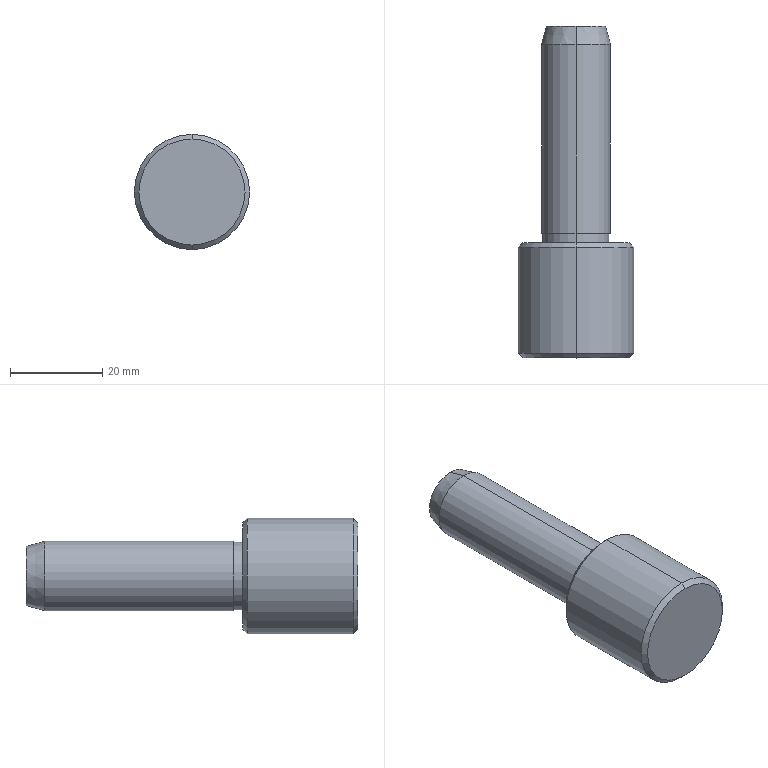Part | STEP file | OP10-024_fix-pin | 1 solid | 16 faces | box 25 x 72 x 25 mm | volume 20386 mm3 | cone 6 | cylinder 6 | plane 4 | commonest cylinder face diameters 14.6 x2 15 x2 25 x2
STEP:
#1=CARTESIAN_POINT('',(0.,0.,0.));
#2=DIRECTION('',(0.,0.,1.));
#3=DIRECTION('',(1.,0.,0.));
#4=AXIS2_PLACEMENT_3D('',#1,#2,#3);
#5=CARTESIAN_POINT('',(0.,72.,6.428));
#6=VERTEX_POINT('',#5);
#7=CARTESIAN_POINT('',(0.,72.,-6.428));
#8=VERTEX_POINT('',#7);
#9=CARTESIAN_POINT('',(0.,72.,0.));
#10=DIRECTION('',(0.,1.,0.));
#11=DIRECTION('',(0.,0.,1.));
#12=AXIS2_PLACEMENT_3D('',#9,#10,#11);
#13=CIRCLE('',#12,6.428);
#14=CARTESIAN_POINT('',(0.,72.,0.));
#15=DIRECTION('',(0.,-1.,0.));
#16=DIRECTION('',(0.,0.,-1.));
#17=AXIS2_PLACEMENT_3D('',#14,#15,#16);
#18=CONICAL_SURFACE('',#17,6.428,0.2618);
#19=CARTESIAN_POINT('',(3.142,0.));
#20=DIRECTION('',(-1.,0.));
#21=VECTOR('',#20,1.);
#22=LINE('',#19,#21);
#23=(GEOMETRIC_REPRESENTATION_CONTEXT(2)PARAMETRIC_REPRESENTATION_CONTEXT()REPRESENTATION_CONTEXT('',''));
#24=DEFINITIONAL_REPRESENTATION('',(#22),#23);
#25=PCURVE('',#18,#24);
#26=CARTESIAN_POINT('',(0.,72.,0.));
#27=DIRECTION('',(0.,1.,0.));
#28=DIRECTION('',(0.,0.,1.));
#29=AXIS2_PLACEMENT_3D('',#26,#27,#28);
#30=PLANE('',#29);
#31=CARTESIAN_POINT('',(0.,0.));
#32=DIRECTION('',(1.,0.));
#33=AXIS2_PLACEMENT_2D('',#31,#32);
#34=CIRCLE('',#33,6.428);
#35=(GEOMETRIC_REPRESENTATION_CONTEXT(2)PARAMETRIC_REPRESENTATION_CONTEXT()REPRESENTATION_CONTEXT('',''));
#36=DEFINITIONAL_REPRESENTATION('',(#34),#35);
#37=PCURVE('',#30,#36);
#38=SURFACE_CURVE('',#13,(#25,#37),.PCURVE_S1.);
#39=EDGE_CURVE('',#6,#8,#38,.T.);
#40=ORIENTED_EDGE('',*,*,#39,.F.);
#41=CARTESIAN_POINT('',(0.,68.,7.5));
#42=VERTEX_POINT('',#41);
#43=CARTESIAN_POINT('',(0.,72.,6.428));
#44=DIRECTION('',(0.,-0.9659,0.2588));
#45=VECTOR('',#44,1.);
#46=LINE('',#43,#45);
#47=CARTESIAN_POINT('',(3.142,0.));
#48=DIRECTION('',(0.,1.));
#49=VECTOR('',#48,1.);
#50=LINE('',#47,#49);
#51=(GEOMETRIC_REPRESENTATION_CONTEXT(2)PARAMETRIC_REPRESENTATION_CONTEXT()REPRESENTATION_CONTEXT('',''));
#52=DEFINITIONAL_REPRESENTATION('',(#50),#51);
#53=PCURVE('',#18,#52);
#54=CARTESIAN_POINT('',(0.,72.,0.));
#55=DIRECTION('',(0.,-1.,0.));
#56=DIRECTION('',(0.,0.,-1.));
#57=AXIS2_PLACEMENT_3D('',#54,#55,#56);
#58=CONICAL_SURFACE('',#57,6.428,0.2618);
#59=CARTESIAN_POINT('',(3.142,0.));
#60=DIRECTION('',(0.,1.));
#61=VECTOR('',#60,1.);
#62=LINE('',#59,#61);
#63=(GEOMETRIC_REPRESENTATION_CONTEXT(2)PARAMETRIC_REPRESENTATION_CONTEXT()REPRESENTATION_CONTEXT('',''));
#64=DEFINITIONAL_REPRESENTATION('',(#62),#63);
#65=PCURVE('',#58,#64);
#66=SURFACE_CURVE('',#46,(#53,#65),.PCURVE_S1.);
#67=EDGE_CURVE('',#6,#42,#66,.T.);
#68=ORIENTED_EDGE('',*,*,#67,.T.);
#69=CARTESIAN_POINT('',(0.,68.,-7.5));
#70=VERTEX_POINT('',#69);
#71=CARTESIAN_POINT('',(0.,68.,0.));
#72=DIRECTION('',(0.,-1.,0.));
#73=DIRECTION('',(0.,0.,1.));
#74=AXIS2_PLACEMENT_3D('',#71,#72,#73);
#75=CIRCLE('',#74,7.5);
#76=CARTESIAN_POINT('',(-3.142,4.));
#77=DIRECTION('',(1.,0.));
#78=VECTOR('',#77,1.);
#79=LINE('',#76,#78);
#80=(GEOMETRIC_REPRESENTATION_CONTEXT(2)PARAMETRIC_REPRESENTATION_CONTEXT()REPRESENTATION_CONTEXT('',''));
#81=DEFINITIONAL_REPRESENTATION('',(#79),#80);
#82=PCURVE('',#18,#81);
#83=CARTESIAN_POINT('',(0.,72.,0.));
#84=DIRECTION('',(0.,-1.,0.));
#85=DIRECTION('',(0.,0.,-1.));
#86=AXIS2_PLACEMENT_3D('',#83,#84,#85);
#87=CYLINDRICAL_SURFACE('',#86,7.5);
#88=CARTESIAN_POINT('',(-3.142,4.));
#89=DIRECTION('',(1.,0.));
#90=VECTOR('',#89,1.);
#91=LINE('',#88,#90);
#92=(GEOMETRIC_REPRESENTATION_CONTEXT(2)PARAMETRIC_REPRESENTATION_CONTEXT()REPRESENTATION_CONTEXT('',''));
#93=DEFINITIONAL_REPRESENTATION('',(#91),#92);
#94=PCURVE('',#87,#93);
#95=SURFACE_CURVE('',#75,(#82,#94),.PCURVE_S1.);
#96=EDGE_CURVE('',#70,#42,#95,.T.);
#97=ORIENTED_EDGE('',*,*,#96,.F.);
#98=CARTESIAN_POINT('',(0.,72.,-6.428));
#99=DIRECTION('',(0.,-0.9659,-0.2588));
#100=VECTOR('',#99,1.);
#101=LINE('',#98,#100);
#102=CARTESIAN_POINT('',(0.,0.));
#103=DIRECTION('',(0.,1.));
#104=VECTOR('',#103,1.);
#105=LINE('',#102,#104);
#106=(GEOMETRIC_REPRESENTATION_CONTEXT(2)PARAMETRIC_REPRESENTATION_CONTEXT()REPRESENTATION_CONTEXT('',''));
#107=DEFINITIONAL_REPRESENTATION('',(#105),#106);
#108=PCURVE('',#18,#107);
#109=CARTESIAN_POINT('',(6.283,0.));
#110=DIRECTION('',(0.,1.));
#111=VECTOR('',#110,1.);
#112=LINE('',#109,#111);
#113=(GEOMETRIC_REPRESENTATION_CONTEXT(2)PARAMETRIC_REPRESENTATION_CONTEXT()REPRESENTATION_CONTEXT('',''));
#114=DEFINITIONAL_REPRESENTATION('',(#112),#113);
#115=PCURVE('',#58,#114);
#116=SURFACE_CURVE('',#101,(#108,#115),.PCURVE_S1.);
#117=EDGE_CURVE('',#8,#70,#116,.T.);
#118=ORIENTED_EDGE('',*,*,#117,.F.);
#119=EDGE_LOOP('',(#40,#68,#97,#118));
#120=FACE_BOUND('',#119,.T.);
#121=ADVANCED_FACE('',(#120),#18,.T.);
#122=ORIENTED_EDGE('',*,*,#96,.T.);
#123=CARTESIAN_POINT('',(0.,27.,7.5));
#124=VERTEX_POINT('',#123);
#125=CARTESIAN_POINT('',(0.,72.,7.5));
#126=DIRECTION('',(0.,-1.,0.));
#127=VECTOR('',#126,1.);
#128=LINE('',#125,#127);
#129=CARTESIAN_POINT('',(3.142,0.));
#130=DIRECTION('',(0.,1.));
#131=VECTOR('',#130,1.);
#132=LINE('',#129,#131);
#133=(GEOMETRIC_REPRESENTATION_CONTEXT(2)PARAMETRIC_REPRESENTATION_CONTEXT()REPRESENTATION_CONTEXT('',''));
#134=DEFINITIONAL_REPRESENTATION('',(#132),#133);
#135=PCURVE('',#87,#134);
#136=CARTESIAN_POINT('',(0.,72.,0.));
#137=DIRECTION('',(0.,-1.,0.));
#138=DIRECTION('',(0.,0.,-1.));
#139=AXIS2_PLACEMENT_3D('',#136,#137,#138);
#140=CYLINDRICAL_SURFACE('',#139,7.5);
#141=CARTESIAN_POINT('',(3.142,0.));
#142=DIRECTION('',(0.,1.));
#143=VECTOR('',#142,1.);
#144=LINE('',#141,#143);
#145=(GEOMETRIC_REPRESENTATION_CONTEXT(2)PARAMETRIC_REPRESENTATION_CONTEXT()REPRESENTATION_CONTEXT('',''));
#146=DEFINITIONAL_REPRESENTATION('',(#144),#145);
#147=PCURVE('',#140,#146);
#148=SURFACE_CURVE('',#128,(#135,#147),.PCURVE_S1.);
#149=EDGE_CURVE('',#42,#124,#148,.T.);
#150=ORIENTED_EDGE('',*,*,#149,.T.);
#151=CARTESIAN_POINT('',(0.,27.,-7.5));
#152=VERTEX_POINT('',#151);
#153=CARTESIAN_POINT('',(0.,27.,0.));
#154=DIRECTION('',(0.,1.,0.));
#155=DIRECTION('',(0.,0.,1.));
#156=AXIS2_PLACEMENT_3D('',#153,#154,#155);
#157=CIRCLE('',#156,7.5);
#158=CARTESIAN_POINT('',(3.142,45.));
#159=DIRECTION('',(-1.,0.));
#160=VECTOR('',#159,1.);
#161=LINE('',#158,#160);
#162=(GEOMETRIC_REPRESENTATION_CONTEXT(2)PARAMETRIC_REPRESENTATION_CONTEXT()REPRESENTATION_CONTEXT('',''));
#163=DEFINITIONAL_REPRESENTATION('',(#161),#162);
#164=PCURVE('',#87,#163);
#165=CARTESIAN_POINT('',(0.,27.,0.));
#166=DIRECTION('',(0.,1.,0.));
#167=DIRECTION('',(0.,0.,1.));
#168=AXIS2_PLACEMENT_3D('',#165,#166,#167);
#169=PLANE('',#168);
#170=CARTESIAN_POINT('',(0.,0.));
#171=DIRECTION('',(1.,0.));
#172=AXIS2_PLACEMENT_2D('',#170,#171);
#173=CIRCLE('',#172,7.5);
#174=(GEOMETRIC_REPRESENTATION_CONTEXT(2)PARAMETRIC_REPRESENTATION_CONTEXT()REPRESENTATION_CONTEXT('',''));
#175=DEFINITIONAL_REPRESENTATION('',(#173),#174);
#176=PCURVE('',#169,#175);
#177=SURFACE_CURVE('',#157,(#164,#176),.PCURVE_S1.);
#178=EDGE_CURVE('',#124,#152,#177,.T.);
#179=ORIENTED_EDGE('',*,*,#178,.T.);
#180=CARTESIAN_POINT('',(0.,72.,-7.5));
#181=DIRECTION('',(0.,-1.,0.));
#182=VECTOR('',#181,1.);
#183=LINE('',#180,#182);
#184=CARTESIAN_POINT('',(0.,0.));
#185=DIRECTION('',(0.,1.));
#186=VECTOR('',#185,1.);
#187=LINE('',#184,#186);
#188=(GEOMETRIC_REPRESENTATION_CONTEXT(2)PARAMETRIC_REPRESENTATION_CONTEXT()REPRESENTATION_CONTEXT('',''));
#189=DEFINITIONAL_REPRESENTATION('',(#187),#188);
#190=PCURVE('',#87,#189);
#191=CARTESIAN_POINT('',(6.283,0.));
#192=DIRECTION('',(0.,1.));
#193=VECTOR('',#192,1.);
#194=LINE('',#191,#193);
#195=(GEOMETRIC_REPRESENTATION_CONTEXT(2)PARAMETRIC_REPRESENTATION_CONTEXT()REPRESENTATION_CONTEXT('',''));
#196=DEFINITIONAL_REPRESENTATION('',(#194),#195);
#197=PCURVE('',#140,#196);
#198=SURFACE_CURVE('',#183,(#190,#197),.PCURVE_S1.);
#199=EDGE_CURVE('',#70,#152,#198,.T.);
#200=ORIENTED_EDGE('',*,*,#199,.F.);
#201=EDGE_LOOP('',(#122,#150,#179,#200));
#202=FACE_BOUND('',#201,.T.);
#203=ADVANCED_FACE('',(#202),#87,.T.);
#204=CARTESIAN_POINT('',(0.,27.,7.3));
#205=VERTEX_POINT('',#204);
#206=CARTESIAN_POINT('',(0.,27.,-7.3));
#207=VERTEX_POINT('',#206);
#208=CARTESIAN_POINT('',(0.,27.,0.));
#209=DIRECTION('',(0.,1.,0.));
#210=DIRECTION('',(0.,0.,1.));
#211=AXIS2_PLACEMENT_3D('',#208,#209,#210);
#212=CIRCLE('',#211,7.3);
#213=CARTESIAN_POINT('',(0.,27.,0.));
#214=DIRECTION('',(0.,-1.,0.));
#215=DIRECTION('',(0.,0.,-1.));
#216=AXIS2_PLACEMENT_3D('',#213,#214,#215);
#217=CYLINDRICAL_SURFACE('',#216,7.3);
#218=CARTESIAN_POINT('',(3.142,0.));
#219=DIRECTION('',(-1.,0.));
#220=VECTOR('',#219,1.);
#221=LINE('',#218,#220);
#222=(GEOMETRIC_REPRESENTATION_CONTEXT(2)PARAMETRIC_REPRESENTATION_CONTEXT()REPRESENTATION_CONTEXT('',''));
#223=DEFINITIONAL_REPRESENTATION('',(#221),#222);
#224=PCURVE('',#217,#223);
#225=CARTESIAN_POINT('',(0.,0.));
#226=DIRECTION('',(1.,0.));
#227=AXIS2_PLACEMENT_2D('',#225,#226);
#228=CIRCLE('',#227,7.3);
#229=(GEOMETRIC_REPRESENTATION_CONTEXT(2)PARAMETRIC_REPRESENTATION_CONTEXT()REPRESENTATION_CONTEXT('',''));
#230=DEFINITIONAL_REPRESENTATION('',(#228),#229);
#231=PCURVE('',#169,#230);
#232=SURFACE_CURVE('',#212,(#224,#231),.PCURVE_S1.);
#233=EDGE_CURVE('',#205,#207,#232,.T.);
#234=ORIENTED_EDGE('',*,*,#233,.F.);
#235=CARTESIAN_POINT('',(0.,25.,7.3));
#236=VERTEX_POINT('',#235);
#237=CARTESIAN_POINT('',(0.,27.,7.3));
#238=DIRECTION('',(0.,-1.,0.));
#239=VECTOR('',#238,1.);
#240=LINE('',#237,#239);
#241=CARTESIAN_POINT('',(3.142,0.));
#242=DIRECTION('',(0.,1.));
#243=VECTOR('',#242,1.);
#244=LINE('',#241,#243);
#245=(GEOMETRIC_REPRESENTATION_CONTEXT(2)PARAMETRIC_REPRESENTATION_CONTEXT()REPRESENTATION_CONTEXT('',''));
#246=DEFINITIONAL_REPRESENTATION('',(#244),#245);
#247=PCURVE('',#217,#246);
#248=CARTESIAN_POINT('',(0.,27.,0.));
#249=DIRECTION('',(0.,-1.,0.));
#250=DIRECTION('',(0.,0.,-1.));
#251=AXIS2_PLACEMENT_3D('',#248,#249,#250);
#252=CYLINDRICAL_SURFACE('',#251,7.3);
#253=CARTESIAN_POINT('',(3.142,0.));
#254=DIRECTION('',(0.,1.));
#255=VECTOR('',#254,1.);
#256=LINE('',#253,#255);
#257=(GEOMETRIC_REPRESENTATION_CONTEXT(2)PARAMETRIC_REPRESENTATION_CONTEXT()REPRESENTATION_CONTEXT('',''));
#258=DEFINITIONAL_REPRESENTATION('',(#256),#257);
#259=PCURVE('',#252,#258);
#260=SURFACE_CURVE('',#240,(#247,#259),.PCURVE_S1.);
#261=EDGE_CURVE('',#205,#236,#260,.T.);
#262=ORIENTED_EDGE('',*,*,#261,.T.);
#263=CARTESIAN_POINT('',(0.,25.,-7.3));
#264=VERTEX_POINT('',#263);
#265=CARTESIAN_POINT('',(0.,25.,0.));
#266=DIRECTION('',(0.,1.,0.));
#267=DIRECTION('',(0.,0.,1.));
#268=AXIS2_PLACEMENT_3D('',#265,#266,#267);
#269=CIRCLE('',#268,7.3);
#270=CARTESIAN_POINT('',(3.142,2.));
#271=DIRECTION('',(-1.,0.));
#272=VECTOR('',#271,1.);
#273=LINE('',#270,#272);
#274=(GEOMETRIC_REPRESENTATION_CONTEXT(2)PARAMETRIC_REPRESENTATION_CONTEXT()REPRESENTATION_CONTEXT('',''));
#275=DEFINITIONAL_REPRESENTATION('',(#273),#274);
#276=PCURVE('',#217,#275);
#277=CARTESIAN_POINT('',(0.,25.,0.));
#278=DIRECTION('',(0.,1.,0.));
#279=DIRECTION('',(0.,0.,1.));
#280=AXIS2_PLACEMENT_3D('',#277,#278,#279);
#281=PLANE('',#280);
#282=CARTESIAN_POINT('',(0.,0.));
#283=DIRECTION('',(1.,0.));
#284=AXIS2_PLACEMENT_2D('',#282,#283);
#285=CIRCLE('',#284,7.3);
#286=(GEOMETRIC_REPRESENTATION_CONTEXT(2)PARAMETRIC_REPRESENTATION_CONTEXT()REPRESENTATION_CONTEXT('',''));
#287=DEFINITIONAL_REPRESENTATION('',(#285),#286);
#288=PCURVE('',#281,#287);
#289=SURFACE_CURVE('',#269,(#276,#288),.PCURVE_S1.);
#290=EDGE_CURVE('',#236,#264,#289,.T.);
#291=ORIENTED_EDGE('',*,*,#290,.T.);
#292=CARTESIAN_POINT('',(0.,27.,-7.3));
#293=DIRECTION('',(0.,-1.,0.));
#294=VECTOR('',#293,1.);
#295=LINE('',#292,#294);
#296=CARTESIAN_POINT('',(0.,0.));
#297=DIRECTION('',(0.,1.));
#298=VECTOR('',#297,1.);
#299=LINE('',#296,#298);
#300=(GEOMETRIC_REPRESENTATION_CONTEXT(2)PARAMETRIC_REPRESENTATION_CONTEXT()REPRESENTATION_CONTEXT('',''));
#301=DEFINITIONAL_REPRESENTATION('',(#299),#300);
#302=PCURVE('',#217,#301);
#303=CARTESIAN_POINT('',(6.283,0.));
#304=DIRECTION('',(0.,1.));
#305=VECTOR('',#304,1.);
#306=LINE('',#303,#305);
#307=(GEOMETRIC_REPRESENTATION_CONTEXT(2)PARAMETRIC_REPRESENTATION_CONTEXT()REPRESENTATION_CONTEXT('',''));
#308=DEFINITIONAL_REPRESENTATION('',(#306),#307);
#309=PCURVE('',#252,#308);
#310=SURFACE_CURVE('',#295,(#302,#309),.PCURVE_S1.);
#311=EDGE_CURVE('',#207,#264,#310,.T.);
#312=ORIENTED_EDGE('',*,*,#311,.F.);
#313=EDGE_LOOP('',(#234,#262,#291,#312));
#314=FACE_BOUND('',#313,.T.);
#315=ADVANCED_FACE('',(#314),#217,.T.);
#316=CARTESIAN_POINT('',(0.,25.,11.5));
#317=VERTEX_POINT('',#316);
#318=CARTESIAN_POINT('',(0.,25.,-11.5));
#319=VERTEX_POINT('',#318);
#320=CARTESIAN_POINT('',(0.,25.,0.));
#321=DIRECTION('',(0.,1.,0.));
#322=DIRECTION('',(0.,0.,1.));
#323=AXIS2_PLACEMENT_3D('',#320,#321,#322);
#324=CIRCLE('',#323,11.5);
#325=CARTESIAN_POINT('',(0.,25.,0.));
#326=DIRECTION('',(0.,-1.,0.));
#327=DIRECTION('',(0.,0.,-1.));
#328=AXIS2_PLACEMENT_3D('',#325,#326,#327);
#329=CONICAL_SURFACE('',#328,11.5,0.7854);
#330=CARTESIAN_POINT('',(3.142,0.));
#331=DIRECTION('',(-1.,0.));
#332=VECTOR('',#331,1.);
#333=LINE('',#330,#332);
#334=(GEOMETRIC_REPRESENTATION_CONTEXT(2)PARAMETRIC_REPRESENTATION_CONTEXT()REPRESENTATION_CONTEXT('',''));
#335=DEFINITIONAL_REPRESENTATION('',(#333),#334);
#336=PCURVE('',#329,#335);
#337=CARTESIAN_POINT('',(0.,0.));
#338=DIRECTION('',(1.,0.));
#339=AXIS2_PLACEMENT_2D('',#337,#338);
#340=CIRCLE('',#339,11.5);
#341=(GEOMETRIC_REPRESENTATION_CONTEXT(2)PARAMETRIC_REPRESENTATION_CONTEXT()REPRESENTATION_CONTEXT('',''));
#342=DEFINITIONAL_REPRESENTATION('',(#340),#341);
#343=PCURVE('',#281,#342);
#344=SURFACE_CURVE('',#324,(#336,#343),.PCURVE_S1.);
#345=EDGE_CURVE('',#317,#319,#344,.T.);
#346=ORIENTED_EDGE('',*,*,#345,.F.);
#347=CARTESIAN_POINT('',(0.,24.,12.5));
#348=VERTEX_POINT('',#347);
#349=CARTESIAN_POINT('',(0.,25.,11.5));
#350=DIRECTION('',(0.,-0.7071,0.7071));
#351=VECTOR('',#350,1.);
#352=LINE('',#349,#351);
#353=CARTESIAN_POINT('',(3.142,0.));
#354=DIRECTION('',(0.,1.));
#355=VECTOR('',#354,1.);
#356=LINE('',#353,#355);
#357=(GEOMETRIC_REPRESENTATION_CONTEXT(2)PARAMETRIC_REPRESENTATION_CONTEXT()REPRESENTATION_CONTEXT('',''));
#358=DEFINITIONAL_REPRESENTATION('',(#356),#357);
#359=PCURVE('',#329,#358);
#360=CARTESIAN_POINT('',(0.,25.,0.));
#361=DIRECTION('',(0.,-1.,0.));
#362=DIRECTION('',(0.,0.,-1.));
#363=AXIS2_PLACEMENT_3D('',#360,#361,#362);
#364=CONICAL_SURFACE('',#363,11.5,0.7854);
#365=CARTESIAN_POINT('',(3.142,0.));
#366=DIRECTION('',(0.,1.));
#367=VECTOR('',#366,1.);
#368=LINE('',#365,#367);
#369=(GEOMETRIC_REPRESENTATION_CONTEXT(2)PARAMETRIC_REPRESENTATION_CONTEXT()REPRESENTATION_CONTEXT('',''));
#370=DEFINITIONAL_REPRESENTATION('',(#368),#369);
#371=PCURVE('',#364,#370);
#372=SURFACE_CURVE('',#352,(#359,#371),.PCURVE_S1.);
#373=EDGE_CURVE('',#317,#348,#372,.T.);
#374=ORIENTED_EDGE('',*,*,#373,.T.);
#375=CARTESIAN_POINT('',(0.,24.,-12.5));
#376=VERTEX_POINT('',#375);
#377=CARTESIAN_POINT('',(0.,24.,0.));
#378=DIRECTION('',(0.,-1.,0.));
#379=DIRECTION('',(0.,0.,1.));
#380=AXIS2_PLACEMENT_3D('',#377,#378,#379);
#381=CIRCLE('',#380,12.5);
#382=CARTESIAN_POINT('',(-3.142,1.));
#383=DIRECTION('',(1.,0.));
#384=VECTOR('',#383,1.);
#385=LINE('',#382,#384);
#386=(GEOMETRIC_REPRESENTATION_CONTEXT(2)PARAMETRIC_REPRESENTATION_CONTEXT()REPRESENTATION_CONTEXT('',''));
#387=DEFINITIONAL_REPRESENTATION('',(#385),#386);
#388=PCURVE('',#329,#387);
#389=CARTESIAN_POINT('',(0.,25.,0.));
#390=DIRECTION('',(0.,-1.,0.));
#391=DIRECTION('',(0.,0.,-1.));
#392=AXIS2_PLACEMENT_3D('',#389,#390,#391);
#393=CYLINDRICAL_SURFACE('',#392,12.5);
#394=CARTESIAN_POINT('',(-3.142,1.));
#395=DIRECTION('',(1.,0.));
#396=VECTOR('',#395,1.);
#397=LINE('',#394,#396);
#398=(GEOMETRIC_REPRESENTATION_CONTEXT(2)PARAMETRIC_REPRESENTATION_CONTEXT()REPRESENTATION_CONTEXT('',''));
#399=DEFINITIONAL_REPRESENTATION('',(#397),#398);
#400=PCURVE('',#393,#399);
#401=SURFACE_CURVE('',#381,(#388,#400),.PCURVE_S1.);
#402=EDGE_CURVE('',#376,#348,#401,.T.);
#403=ORIENTED_EDGE('',*,*,#402,.F.);
#404=CARTESIAN_POINT('',(0.,25.,-11.5));
#405=DIRECTION('',(0.,-0.7071,-0.7071));
#406=VECTOR('',#405,1.);
#407=LINE('',#404,#406);
#408=CARTESIAN_POINT('',(0.,0.));
#409=DIRECTION('',(0.,1.));
#410=VECTOR('',#409,1.);
#411=LINE('',#408,#410);
#412=(GEOMETRIC_REPRESENTATION_CONTEXT(2)PARAMETRIC_REPRESENTATION_CONTEXT()REPRESENTATION_CONTEXT('',''));
#413=DEFINITIONAL_REPRESENTATION('',(#411),#412);
#414=PCURVE('',#329,#413);
#415=CARTESIAN_POINT('',(6.283,0.));
#416=DIRECTION('',(0.,1.));
#417=VECTOR('',#416,1.);
#418=LINE('',#415,#417);
#419=(GEOMETRIC_REPRESENTATION_CONTEXT(2)PARAMETRIC_REPRESENTATION_CONTEXT()REPRESENTATION_CONTEXT('',''));
#420=DEFINITIONAL_REPRESENTATION('',(#418),#419);
#421=PCURVE('',#364,#420);
#422=SURFACE_CURVE('',#407,(#414,#421),.PCURVE_S1.);
#423=EDGE_CURVE('',#319,#376,#422,.T.);
#424=ORIENTED_EDGE('',*,*,#423,.F.);
#425=EDGE_LOOP('',(#346,#374,#403,#424));
#426=FACE_BOUND('',#425,.T.);
#427=ADVANCED_FACE('',(#426),#329,.T.);
#428=CARTESIAN_POINT('',(0.,0.,-11.5));
#429=VERTEX_POINT('',#428);
#430=CARTESIAN_POINT('',(0.,0.,11.5));
#431=VERTEX_POINT('',#430);
#432=CARTESIAN_POINT('',(0.,0.,0.));
#433=DIRECTION('',(0.,-1.,0.));
#434=DIRECTION('',(0.,0.,1.));
#435=AXIS2_PLACEMENT_3D('',#432,#433,#434);
#436=CIRCLE('',#435,11.5);
#437=CARTESIAN_POINT('',(0.,1.,0.));
#438=DIRECTION('',(0.,1.,0.));
#439=DIRECTION('',(0.,0.,1.));
#440=AXIS2_PLACEMENT_3D('',#437,#438,#439);
#441=CONICAL_SURFACE('',#440,12.5,0.7854);
#442=CARTESIAN_POINT('',(6.283,-1.));
#443=DIRECTION('',(-1.,0.));
#444=VECTOR('',#443,1.);
#445=LINE('',#442,#444);
#446=(GEOMETRIC_REPRESENTATION_CONTEXT(2)PARAMETRIC_REPRESENTATION_CONTEXT()REPRESENTATION_CONTEXT('',''));
#447=DEFINITIONAL_REPRESENTATION('',(#445),#446);
#448=PCURVE('',#441,#447);
#449=CARTESIAN_POINT('',(0.,0.,0.));
#450=DIRECTION('',(0.,1.,0.));
#451=DIRECTION('',(0.,0.,1.));
#452=AXIS2_PLACEMENT_3D('',#449,#450,#451);
#453=PLANE('',#452);
#454=CARTESIAN_POINT('',(11.5,0.));
#455=CARTESIAN_POINT('',(11.5,-19.919));
#456=CARTESIAN_POINT('',(-5.75,-9.959));
#457=CARTESIAN_POINT('',(-23.,0.));
#458=CARTESIAN_POINT('',(-5.75,9.959));
#459=CARTESIAN_POINT('',(11.5,19.919));
#460=CARTESIAN_POINT('',(11.5,0.));
#461=(BOUNDED_CURVE()B_SPLINE_CURVE(2,(#454,#455,#456,#457,#458,#459,#460),.UNSPECIFIED.,.T.,.F.)B_SPLINE_CURVE_WITH_KNOTS((1,2,2,2,2,1),(-2.094,0.,2.094,4.189,6.283,8.378),.UNSPECIFIED.)CURVE()GEOMETRIC_REPRESENTATION_ITEM()RATIONAL_B_SPLINE_CURVE((1.,0.5,1.,0.5,1.,0.5,1.))REPRESENTATION_ITEM(''));
#462=(GEOMETRIC_REPRESENTATION_CONTEXT(2)PARAMETRIC_REPRESENTATION_CONTEXT()REPRESENTATION_CONTEXT('',''));
#463=DEFINITIONAL_REPRESENTATION('',(#461),#462);
#464=PCURVE('',#453,#463);
#465=SURFACE_CURVE('',#436,(#448,#464),.PCURVE_S1.);
#466=EDGE_CURVE('',#429,#431,#465,.T.);
#467=ORIENTED_EDGE('',*,*,#466,.F.);
#468=CARTESIAN_POINT('',(0.,1.,-12.5));
#469=VERTEX_POINT('',#468);
#470=CARTESIAN_POINT('',(0.,1.,-12.5));
#471=DIRECTION('',(0.,0.7071,-0.7071));
#472=VECTOR('',#471,1.);
#473=LINE('',#470,#472);
#474=CARTESIAN_POINT('',(3.142,0.));
#475=DIRECTION('',(0.,1.));
#476=VECTOR('',#475,1.);
#477=LINE('',#474,#476);
#478=(GEOMETRIC_REPRESENTATION_CONTEXT(2)PARAMETRIC_REPRESENTATION_CONTEXT()REPRESENTATION_CONTEXT('',''));
#479=DEFINITIONAL_REPRESENTATION('',(#477),#478);
#480=PCURVE('',#441,#479);
#481=CARTESIAN_POINT('',(0.,1.,0.));
#482=DIRECTION('',(0.,1.,0.));
#483=DIRECTION('',(0.,0.,1.));
#484=AXIS2_PLACEMENT_3D('',#481,#482,#483);
#485=CONICAL_SURFACE('',#484,12.5,0.7854);
#486=CARTESIAN_POINT('',(3.142,0.));
#487=DIRECTION('',(0.,1.));
#488=VECTOR('',#487,1.);
#489=LINE('',#486,#488);
#490=(GEOMETRIC_REPRESENTATION_CONTEXT(2)PARAMETRIC_REPRESENTATION_CONTEXT()REPRESENTATION_CONTEXT('',''));
#491=DEFINITIONAL_REPRESENTATION('',(#489),#490);
#492=PCURVE('',#485,#491);
#493=SURFACE_CURVE('',#473,(#480,#492),.PCURVE_S1.);
#494=EDGE_CURVE('',#429,#469,#493,.T.);
#495=ORIENTED_EDGE('',*,*,#494,.T.);
#496=CARTESIAN_POINT('',(0.,1.,12.5));
#497=VERTEX_POINT('',#496);
#498=CARTESIAN_POINT('',(0.,1.,0.));
#499=DIRECTION('',(0.,1.,0.));
#500=DIRECTION('',(0.,0.,1.));
#501=AXIS2_PLACEMENT_3D('',#498,#499,#500);
#502=CIRCLE('',#501,12.5);
#503=CARTESIAN_POINT('',(0.,0.));
#504=DIRECTION('',(1.,0.));
#505=VECTOR('',#504,1.);
#506=LINE('',#503,#505);
#507=(GEOMETRIC_REPRESENTATION_CONTEXT(2)PARAMETRIC_REPRESENTATION_CONTEXT()REPRESENTATION_CONTEXT('',''));
#508=DEFINITIONAL_REPRESENTATION('',(#506),#507);
#509=PCURVE('',#441,#508);
#510=CARTESIAN_POINT('',(3.142,24.));
#511=DIRECTION('',(-1.,0.));
#512=VECTOR('',#511,1.);
#513=LINE('',#510,#512);
#514=(GEOMETRIC_REPRESENTATION_CONTEXT(2)PARAMETRIC_REPRESENTATION_CONTEXT()REPRESENTATION_CONTEXT('',''));
#515=DEFINITIONAL_REPRESENTATION('',(#513),#514);
#516=PCURVE('',#393,#515);
#517=SURFACE_CURVE('',#502,(#509,#516),.PCURVE_S1.);
#518=EDGE_CURVE('',#497,#469,#517,.T.);
#519=ORIENTED_EDGE('',*,*,#518,.F.);
#520=CARTESIAN_POINT('',(0.,1.,12.5));
#521=DIRECTION('',(0.,0.7071,0.7071));
#522=VECTOR('',#521,1.);
#523=LINE('',#520,#522);
#524=CARTESIAN_POINT('',(0.,0.));
#525=DIRECTION('',(0.,1.));
#526=VECTOR('',#525,1.);
#527=LINE('',#524,#526);
#528=(GEOMETRIC_REPRESENTATION_CONTEXT(2)PARAMETRIC_REPRESENTATION_CONTEXT()REPRESENTATION_CONTEXT('',''));
#529=DEFINITIONAL_REPRESENTATION('',(#527),#528);
#530=PCURVE('',#441,#529);
#531=CARTESIAN_POINT('',(6.283,0.));
#532=DIRECTION('',(0.,1.));
#533=VECTOR('',#532,1.);
#534=LINE('',#531,#533);
#535=(GEOMETRIC_REPRESENTATION_CONTEXT(2)PARAMETRIC_REPRESENTATION_CONTEXT()REPRESENTATION_CONTEXT('',''));
#536=DEFINITIONAL_REPRESENTATION('',(#534),#535);
#537=PCURVE('',#485,#536);
#538=SURFACE_CURVE('',#523,(#530,#537),.PCURVE_S1.);
#539=EDGE_CURVE('',#431,#497,#538,.T.);
#540=ORIENTED_EDGE('',*,*,#539,.F.);
#541=EDGE_LOOP('',(#467,#495,#519,#540));
#542=FACE_BOUND('',#541,.T.);
#543=ADVANCED_FACE('',(#542),#441,.T.);
#544=ORIENTED_EDGE('',*,*,#402,.T.);
#545=CARTESIAN_POINT('',(0.,25.,12.5));
#546=DIRECTION('',(0.,-1.,0.));
#547=VECTOR('',#546,1.);
#548=LINE('',#545,#547);
#549=CARTESIAN_POINT('',(3.142,0.));
#550=DIRECTION('',(0.,1.));
#551=VECTOR('',#550,1.);
#552=LINE('',#549,#551);
#553=(GEOMETRIC_REPRESENTATION_CONTEXT(2)PARAMETRIC_REPRESENTATION_CONTEXT()REPRESENTATION_CONTEXT('',''));
#554=DEFINITIONAL_REPRESENTATION('',(#552),#553);
#555=PCURVE('',#393,#554);
#556=CARTESIAN_POINT('',(0.,25.,0.));
#557=DIRECTION('',(0.,-1.,0.));
#558=DIRECTION('',(0.,0.,-1.));
#559=AXIS2_PLACEMENT_3D('',#556,#557,#558);
#560=CYLINDRICAL_SURFACE('',#559,12.5);
#561=CARTESIAN_POINT('',(3.142,0.));
#562=DIRECTION('',(0.,1.));
#563=VECTOR('',#562,1.);
#564=LINE('',#561,#563);
#565=(GEOMETRIC_REPRESENTATION_CONTEXT(2)PARAMETRIC_REPRESENTATION_CONTEXT()REPRESENTATION_CONTEXT('',''));
#566=DEFINITIONAL_REPRESENTATION('',(#564),#565);
#567=PCURVE('',#560,#566);
#568=SURFACE_CURVE('',#548,(#555,#567),.PCURVE_S1.);
#569=EDGE_CURVE('',#348,#497,#568,.T.);
#570=ORIENTED_EDGE('',*,*,#569,.T.);
#571=ORIENTED_EDGE('',*,*,#518,.T.);
#572=CARTESIAN_POINT('',(0.,25.,-12.5));
#573=DIRECTION('',(0.,-1.,0.));
#574=VECTOR('',#573,1.);
#575=LINE('',#572,#574);
#576=CARTESIAN_POINT('',(0.,0.));
#577=DIRECTION('',(0.,1.));
#578=VECTOR('',#577,1.);
#579=LINE('',#576,#578);
#580=(GEOMETRIC_REPRESENTATION_CONTEXT(2)PARAMETRIC_REPRESENTATION_CONTEXT()REPRESENTATION_CONTEXT('',''));
#581=DEFINITIONAL_REPRESENTATION('',(#579),#580);
#582=PCURVE('',#393,#581);
#583=CARTESIAN_POINT('',(6.283,0.));
#584=DIRECTION('',(0.,1.));
#585=VECTOR('',#584,1.);
#586=LINE('',#583,#585);
#587=(GEOMETRIC_REPRESENTATION_CONTEXT(2)PARAMETRIC_REPRESENTATION_CONTEXT()REPRESENTATION_CONTEXT('',''));
#588=DEFINITIONAL_REPRESENTATION('',(#586),#587);
#589=PCURVE('',#560,#588);
#590=SURFACE_CURVE('',#575,(#582,#589),.PCURVE_S1.);
#591=EDGE_CURVE('',#376,#469,#590,.T.);
#592=ORIENTED_EDGE('',*,*,#591,.F.);
#593=EDGE_LOOP('',(#544,#570,#571,#592));
#594=FACE_BOUND('',#593,.T.);
#595=ADVANCED_FACE('',(#594),#393,.T.);
#596=CARTESIAN_POINT('',(0.,25.,0.));
#597=DIRECTION('',(0.,1.,0.));
#598=DIRECTION('',(0.,0.,1.));
#599=AXIS2_PLACEMENT_3D('',#596,#597,#598);
#600=CIRCLE('',#599,7.3);
#601=CARTESIAN_POINT('',(0.,0.));
#602=DIRECTION('',(1.,0.));
#603=AXIS2_PLACEMENT_2D('',#601,#602);
#604=CIRCLE('',#603,7.3);
#605=(GEOMETRIC_REPRESENTATION_CONTEXT(2)PARAMETRIC_REPRESENTATION_CONTEXT()REPRESENTATION_CONTEXT('',''));
#606=DEFINITIONAL_REPRESENTATION('',(#604),#605);
#607=PCURVE('',#281,#606);
#608=CARTESIAN_POINT('',(9.425,2.));
#609=DIRECTION('',(-1.,0.));
#610=VECTOR('',#609,1.);
#611=LINE('',#608,#610);
#612=(GEOMETRIC_REPRESENTATION_CONTEXT(2)PARAMETRIC_REPRESENTATION_CONTEXT()REPRESENTATION_CONTEXT('',''));
#613=DEFINITIONAL_REPRESENTATION('',(#611),#612);
#614=PCURVE('',#252,#613);
#615=SURFACE_CURVE('',#600,(#607,#614),.PCURVE_S1.);
#616=EDGE_CURVE('',#264,#236,#615,.T.);
#617=ORIENTED_EDGE('',*,*,#616,.F.);
#618=ORIENTED_EDGE('',*,*,#290,.F.);
#619=EDGE_LOOP('',(#617,#618));
#620=FACE_BOUND('',#619,.T.);
#621=CARTESIAN_POINT('',(0.,25.,0.));
#622=DIRECTION('',(0.,1.,0.));
#623=DIRECTION('',(0.,0.,1.));
#624=AXIS2_PLACEMENT_3D('',#621,#622,#623);
#625=CIRCLE('',#624,11.5);
#626=CARTESIAN_POINT('',(0.,0.));
#627=DIRECTION('',(1.,0.));
#628=AXIS2_PLACEMENT_2D('',#626,#627);
#629=CIRCLE('',#628,11.5);
#630=(GEOMETRIC_REPRESENTATION_CONTEXT(2)PARAMETRIC_REPRESENTATION_CONTEXT()REPRESENTATION_CONTEXT('',''));
#631=DEFINITIONAL_REPRESENTATION('',(#629),#630);
#632=PCURVE('',#281,#631);
#633=CARTESIAN_POINT('',(9.425,0.));
#634=DIRECTION('',(-1.,0.));
#635=VECTOR('',#634,1.);
#636=LINE('',#633,#635);
#637=(GEOMETRIC_REPRESENTATION_CONTEXT(2)PARAMETRIC_REPRESENTATION_CONTEXT()REPRESENTATION_CONTEXT('',''));
#638=DEFINITIONAL_REPRESENTATION('',(#636),#637);
#639=PCURVE('',#364,#638);
#640=SURFACE_CURVE('',#625,(#632,#639),.PCURVE_S1.);
#641=EDGE_CURVE('',#319,#317,#640,.T.);
#642=ORIENTED_EDGE('',*,*,#641,.T.);
#643=ORIENTED_EDGE('',*,*,#345,.T.);
#644=EDGE_LOOP('',(#642,#643));
#645=FACE_BOUND('',#644,.T.);
#646=ADVANCED_FACE('',(#620,#645),#281,.T.);
#647=ORIENTED_EDGE('',*,*,#569,.F.);
#648=CARTESIAN_POINT('',(0.,24.,0.));
#649=DIRECTION('',(0.,-1.,0.));
#650=DIRECTION('',(0.,0.,1.));
#651=AXIS2_PLACEMENT_3D('',#648,#649,#650);
#652=CIRCLE('',#651,12.5);
#653=CARTESIAN_POINT('',(3.142,1.));
#654=DIRECTION('',(1.,0.));
#655=VECTOR('',#654,1.);
#656=LINE('',#653,#655);
#657=(GEOMETRIC_REPRESENTATION_CONTEXT(2)PARAMETRIC_REPRESENTATION_CONTEXT()REPRESENTATION_CONTEXT('',''));
#658=DEFINITIONAL_REPRESENTATION('',(#656),#657);
#659=PCURVE('',#560,#658);
#660=CARTESIAN_POINT('',(3.142,1.));
#661=DIRECTION('',(1.,0.));
#662=VECTOR('',#661,1.);
#663=LINE('',#660,#662);
#664=(GEOMETRIC_REPRESENTATION_CONTEXT(2)PARAMETRIC_REPRESENTATION_CONTEXT()REPRESENTATION_CONTEXT('',''));
#665=DEFINITIONAL_REPRESENTATION('',(#663),#664);
#666=PCURVE('',#364,#665);
#667=SURFACE_CURVE('',#652,(#659,#666),.PCURVE_S1.);
#668=EDGE_CURVE('',#348,#376,#667,.T.);
#669=ORIENTED_EDGE('',*,*,#668,.T.);
#670=ORIENTED_EDGE('',*,*,#591,.T.);
#671=CARTESIAN_POINT('',(0.,1.,0.));
#672=DIRECTION('',(0.,1.,0.));
#673=DIRECTION('',(0.,0.,1.));
#674=AXIS2_PLACEMENT_3D('',#671,#672,#673);
#675=CIRCLE('',#674,12.5);
#676=CARTESIAN_POINT('',(9.425,24.));
#677=DIRECTION('',(-1.,0.));
#678=VECTOR('',#677,1.);
#679=LINE('',#676,#678);
#680=(GEOMETRIC_REPRESENTATION_CONTEXT(2)PARAMETRIC_REPRESENTATION_CONTEXT()REPRESENTATION_CONTEXT('',''));
#681=DEFINITIONAL_REPRESENTATION('',(#679),#680);
#682=PCURVE('',#560,#681);
#683=CARTESIAN_POINT('',(0.,0.));
#684=DIRECTION('',(1.,0.));
#685=VECTOR('',#684,1.);
#686=LINE('',#683,#685);
#687=(GEOMETRIC_REPRESENTATION_CONTEXT(2)PARAMETRIC_REPRESENTATION_CONTEXT()REPRESENTATION_CONTEXT('',''));
#688=DEFINITIONAL_REPRESENTATION('',(#686),#687);
#689=PCURVE('',#485,#688);
#690=SURFACE_CURVE('',#675,(#682,#689),.PCURVE_S1.);
#691=EDGE_CURVE('',#469,#497,#690,.T.);
#692=ORIENTED_EDGE('',*,*,#691,.T.);
#693=EDGE_LOOP('',(#647,#669,#670,#692));
#694=FACE_BOUND('',#693,.T.);
#695=ADVANCED_FACE('',(#694),#560,.T.);
#696=CARTESIAN_POINT('',(0.,0.,0.));
#697=DIRECTION('',(0.,-1.,0.));
#698=DIRECTION('',(0.,0.,1.));
#699=AXIS2_PLACEMENT_3D('',#696,#697,#698);
#700=CIRCLE('',#699,11.5);
#701=CARTESIAN_POINT('',(11.5,0.));
#702=CARTESIAN_POINT('',(11.5,-19.919));
#703=CARTESIAN_POINT('',(-5.75,-9.959));
#704=CARTESIAN_POINT('',(-23.,0.));
#705=CARTESIAN_POINT('',(-5.75,9.959));
#706=CARTESIAN_POINT('',(11.5,19.919));
#707=CARTESIAN_POINT('',(11.5,0.));
#708=(BOUNDED_CURVE()B_SPLINE_CURVE(2,(#701,#702,#703,#704,#705,#706,#707),.UNSPECIFIED.,.T.,.F.)B_SPLINE_CURVE_WITH_KNOTS((1,2,2,2,2,1),(-2.094,0.,2.094,4.189,6.283,8.378),.UNSPECIFIED.)CURVE()GEOMETRIC_REPRESENTATION_ITEM()RATIONAL_B_SPLINE_CURVE((1.,0.5,1.,0.5,1.,0.5,1.))REPRESENTATION_ITEM(''));
#709=(GEOMETRIC_REPRESENTATION_CONTEXT(2)PARAMETRIC_REPRESENTATION_CONTEXT()REPRESENTATION_CONTEXT('',''));
#710=DEFINITIONAL_REPRESENTATION('',(#708),#709);
#711=PCURVE('',#453,#710);
#712=CARTESIAN_POINT('',(6.283,-1.));
#713=DIRECTION('',(-1.,0.));
#714=VECTOR('',#713,1.);
#715=LINE('',#712,#714);
#716=(GEOMETRIC_REPRESENTATION_CONTEXT(2)PARAMETRIC_REPRESENTATION_CONTEXT()REPRESENTATION_CONTEXT('',''));
#717=DEFINITIONAL_REPRESENTATION('',(#715),#716);
#718=PCURVE('',#485,#717);
#719=SURFACE_CURVE('',#700,(#711,#718),.PCURVE_S1.);
#720=EDGE_CURVE('',#431,#429,#719,.T.);
#721=ORIENTED_EDGE('',*,*,#720,.T.);
#722=ORIENTED_EDGE('',*,*,#466,.T.);
#723=EDGE_LOOP('',(#721,#722));
#724=FACE_BOUND('',#723,.T.);
#725=ADVANCED_FACE('',(#724),#453,.F.);
#726=ORIENTED_EDGE('',*,*,#494,.F.);
#727=ORIENTED_EDGE('',*,*,#720,.F.);
#728=ORIENTED_EDGE('',*,*,#539,.T.);
#729=ORIENTED_EDGE('',*,*,#691,.F.);
#730=EDGE_LOOP('',(#726,#727,#728,#729));
#731=FACE_BOUND('',#730,.T.);
#732=ADVANCED_FACE('',(#731),#485,.T.);
#733=ORIENTED_EDGE('',*,*,#373,.F.);
#734=ORIENTED_EDGE('',*,*,#641,.F.);
#735=ORIENTED_EDGE('',*,*,#423,.T.);
#736=ORIENTED_EDGE('',*,*,#668,.F.);
#737=EDGE_LOOP('',(#733,#734,#735,#736));
#738=FACE_BOUND('',#737,.T.);
#739=ADVANCED_FACE('',(#738),#364,.T.);
#740=CARTESIAN_POINT('',(0.,27.,0.));
#741=DIRECTION('',(0.,1.,0.));
#742=DIRECTION('',(0.,0.,1.));
#743=AXIS2_PLACEMENT_3D('',#740,#741,#742);
#744=CIRCLE('',#743,7.3);
#745=CARTESIAN_POINT('',(0.,0.));
#746=DIRECTION('',(1.,0.));
#747=AXIS2_PLACEMENT_2D('',#745,#746);
#748=CIRCLE('',#747,7.3);
#749=(GEOMETRIC_REPRESENTATION_CONTEXT(2)PARAMETRIC_REPRESENTATION_CONTEXT()REPRESENTATION_CONTEXT('',''));
#750=DEFINITIONAL_REPRESENTATION('',(#748),#749);
#751=PCURVE('',#169,#750);
#752=CARTESIAN_POINT('',(9.425,0.));
#753=DIRECTION('',(-1.,0.));
#754=VECTOR('',#753,1.);
#755=LINE('',#752,#754);
#756=(GEOMETRIC_REPRESENTATION_CONTEXT(2)PARAMETRIC_REPRESENTATION_CONTEXT()REPRESENTATION_CONTEXT('',''));
#757=DEFINITIONAL_REPRESENTATION('',(#755),#756);
#758=PCURVE('',#252,#757);
#759=SURFACE_CURVE('',#744,(#751,#758),.PCURVE_S1.);
#760=EDGE_CURVE('',#207,#205,#759,.T.);
#761=ORIENTED_EDGE('',*,*,#760,.T.);
#762=ORIENTED_EDGE('',*,*,#233,.T.);
#763=EDGE_LOOP('',(#761,#762));
#764=FACE_BOUND('',#763,.T.);
#765=CARTESIAN_POINT('',(0.,27.,0.));
#766=DIRECTION('',(0.,1.,0.));
#767=DIRECTION('',(0.,0.,1.));
#768=AXIS2_PLACEMENT_3D('',#765,#766,#767);
#769=CIRCLE('',#768,7.5);
#770=CARTESIAN_POINT('',(0.,0.));
#771=DIRECTION('',(1.,0.));
#772=AXIS2_PLACEMENT_2D('',#770,#771);
#773=CIRCLE('',#772,7.5);
#774=(GEOMETRIC_REPRESENTATION_CONTEXT(2)PARAMETRIC_REPRESENTATION_CONTEXT()REPRESENTATION_CONTEXT('',''));
#775=DEFINITIONAL_REPRESENTATION('',(#773),#774);
#776=PCURVE('',#169,#775);
#777=CARTESIAN_POINT('',(9.425,45.));
#778=DIRECTION('',(-1.,0.));
#779=VECTOR('',#778,1.);
#780=LINE('',#777,#779);
#781=(GEOMETRIC_REPRESENTATION_CONTEXT(2)PARAMETRIC_REPRESENTATION_CONTEXT()REPRESENTATION_CONTEXT('',''));
#782=DEFINITIONAL_REPRESENTATION('',(#780),#781);
#783=PCURVE('',#140,#782);
#784=SURFACE_CURVE('',#769,(#776,#783),.PCURVE_S1.);
#785=EDGE_CURVE('',#152,#124,#784,.T.);
#786=ORIENTED_EDGE('',*,*,#785,.F.);
#787=ORIENTED_EDGE('',*,*,#178,.F.);
#788=EDGE_LOOP('',(#786,#787));
#789=FACE_BOUND('',#788,.T.);
#790=ADVANCED_FACE('',(#764,#789),#169,.F.);
#791=ORIENTED_EDGE('',*,*,#261,.F.);
#792=ORIENTED_EDGE('',*,*,#760,.F.);
#793=ORIENTED_EDGE('',*,*,#311,.T.);
#794=ORIENTED_EDGE('',*,*,#616,.T.);
#795=EDGE_LOOP('',(#791,#792,#793,#794));
#796=FACE_BOUND('',#795,.T.);
#797=ADVANCED_FACE('',(#796),#252,.T.);
#798=CARTESIAN_POINT('',(0.,72.,0.));
#799=DIRECTION('',(0.,1.,0.));
#800=DIRECTION('',(0.,0.,1.));
#801=AXIS2_PLACEMENT_3D('',#798,#799,#800);
#802=CIRCLE('',#801,6.428);
#803=CARTESIAN_POINT('',(0.,0.));
#804=DIRECTION('',(1.,0.));
#805=AXIS2_PLACEMENT_2D('',#803,#804);
#806=CIRCLE('',#805,6.428);
#807=(GEOMETRIC_REPRESENTATION_CONTEXT(2)PARAMETRIC_REPRESENTATION_CONTEXT()REPRESENTATION_CONTEXT('',''));
#808=DEFINITIONAL_REPRESENTATION('',(#806),#807);
#809=PCURVE('',#30,#808);
#810=CARTESIAN_POINT('',(9.425,0.));
#811=DIRECTION('',(-1.,0.));
#812=VECTOR('',#811,1.);
#813=LINE('',#810,#812);
#814=(GEOMETRIC_REPRESENTATION_CONTEXT(2)PARAMETRIC_REPRESENTATION_CONTEXT()REPRESENTATION_CONTEXT('',''));
#815=DEFINITIONAL_REPRESENTATION('',(#813),#814);
#816=PCURVE('',#58,#815);
#817=SURFACE_CURVE('',#802,(#809,#816),.PCURVE_S1.);
#818=EDGE_CURVE('',#8,#6,#817,.T.);
#819=ORIENTED_EDGE('',*,*,#818,.T.);
#820=ORIENTED_EDGE('',*,*,#39,.T.);
#821=EDGE_LOOP('',(#819,#820));
#822=FACE_BOUND('',#821,.T.);
#823=ADVANCED_FACE('',(#822),#30,.T.);
#824=ORIENTED_EDGE('',*,*,#149,.F.);
#825=CARTESIAN_POINT('',(0.,68.,0.));
#826=DIRECTION('',(0.,-1.,0.));
#827=DIRECTION('',(0.,0.,1.));
#828=AXIS2_PLACEMENT_3D('',#825,#826,#827);
#829=CIRCLE('',#828,7.5);
#830=CARTESIAN_POINT('',(3.142,4.));
#831=DIRECTION('',(1.,0.));
#832=VECTOR('',#831,1.);
#833=LINE('',#830,#832);
#834=(GEOMETRIC_REPRESENTATION_CONTEXT(2)PARAMETRIC_REPRESENTATION_CONTEXT()REPRESENTATION_CONTEXT('',''));
#835=DEFINITIONAL_REPRESENTATION('',(#833),#834);
#836=PCURVE('',#140,#835);
#837=CARTESIAN_POINT('',(3.142,4.));
#838=DIRECTION('',(1.,0.));
#839=VECTOR('',#838,1.);
#840=LINE('',#837,#839);
#841=(GEOMETRIC_REPRESENTATION_CONTEXT(2)PARAMETRIC_REPRESENTATION_CONTEXT()REPRESENTATION_CONTEXT('',''));
#842=DEFINITIONAL_REPRESENTATION('',(#840),#841);
#843=PCURVE('',#58,#842);
#844=SURFACE_CURVE('',#829,(#836,#843),.PCURVE_S1.);
#845=EDGE_CURVE('',#42,#70,#844,.T.);
#846=ORIENTED_EDGE('',*,*,#845,.T.);
#847=ORIENTED_EDGE('',*,*,#199,.T.);
#848=ORIENTED_EDGE('',*,*,#785,.T.);
#849=EDGE_LOOP('',(#824,#846,#847,#848));
#850=FACE_BOUND('',#849,.T.);
#851=ADVANCED_FACE('',(#850),#140,.T.);
#852=ORIENTED_EDGE('',*,*,#67,.F.);
#853=ORIENTED_EDGE('',*,*,#818,.F.);
#854=ORIENTED_EDGE('',*,*,#117,.T.);
#855=ORIENTED_EDGE('',*,*,#845,.F.);
#856=EDGE_LOOP('',(#852,#853,#854,#855));
#857=FACE_BOUND('',#856,.T.);
#858=ADVANCED_FACE('',(#857),#58,.T.);
#859=CLOSED_SHELL('',(#121,#203,#315,#427,#543,#595,#646,#695,#725,#732,#739,#790,#797,#823,#851,#858));
#860=MANIFOLD_SOLID_BREP('',#859);
#861=(LENGTH_UNIT()NAMED_UNIT(*)SI_UNIT(.MILLI.,.METRE.));
#862=UNCERTAINTY_MEASURE_WITH_UNIT(LENGTH_MEASURE(0.0000001),#861,'','');
#863=(NAMED_UNIT(*)PLANE_ANGLE_UNIT()SI_UNIT($,.RADIAN.));
#864=(NAMED_UNIT(*)SI_UNIT($,.STERADIAN.)SOLID_ANGLE_UNIT());
#865=(GEOMETRIC_REPRESENTATION_CONTEXT(3)GLOBAL_UNCERTAINTY_ASSIGNED_CONTEXT((#862))GLOBAL_UNIT_ASSIGNED_CONTEXT((#861,#863,#864))REPRESENTATION_CONTEXT('',''));
#866=ADVANCED_BREP_SHAPE_REPRESENTATION('',(#4,#860),#865);